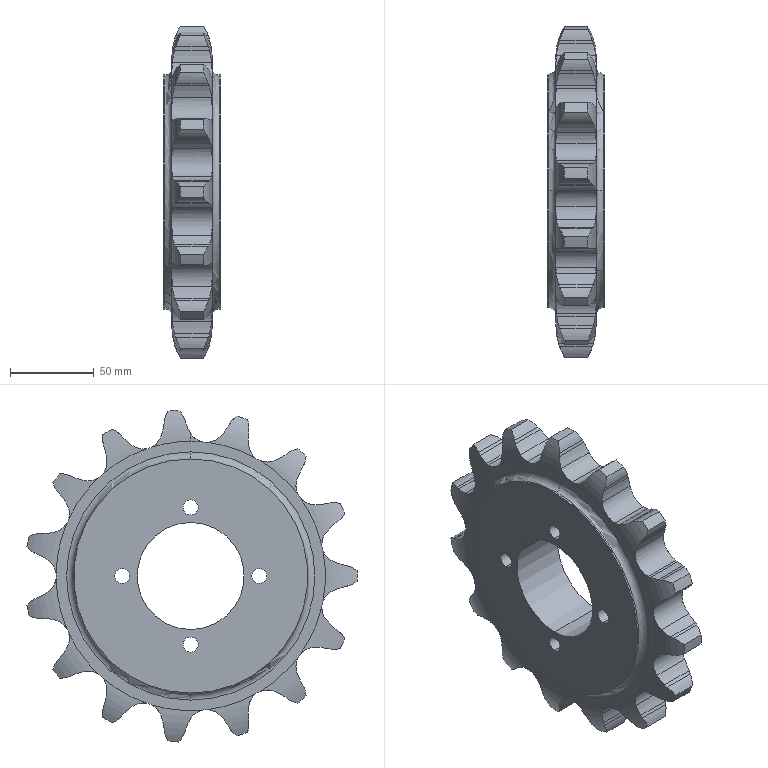Part | SolidWorks | features ICE 3, CirPattern 1, Cut 1, HoleWzd 1, RefAxis 1, Revolution 1 | 1 solid | 193 faces | box 34.469 x 197.46 x 198.492 mm | volume 621986 mm3 | cylinder 119 | plane 38 | torus 36 | commonest cylinder face diameters 32.838 x32 58.009 x31 22.441 x19 199 x15 9 x8 15 x8